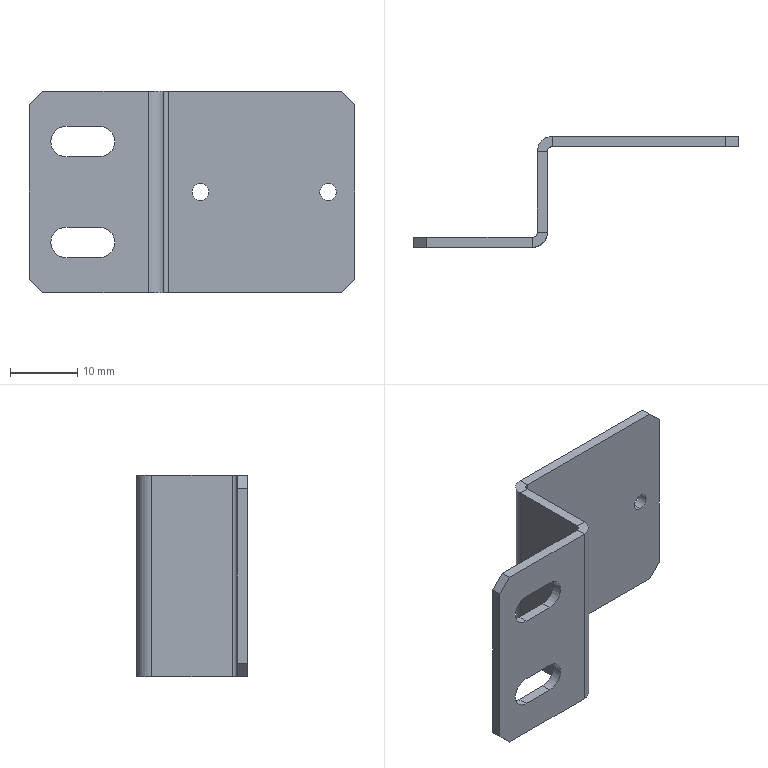Part | STEP file | PN_0044 | 1 solid | 40 faces | box 48.5 x 16.5 x 30 mm | volume 2658 mm3 | plane 26 | cylinder 14 | commonest cylinder face diameters 4.5 x6 2.5 x4 1.473 x2 4.473 x2